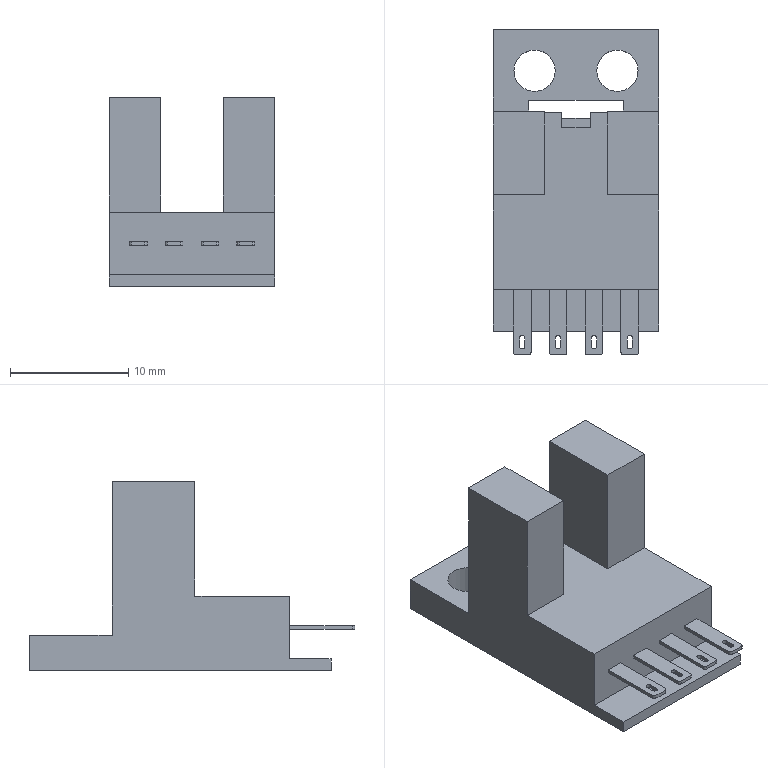Part | NX | 1 solid | 75 faces | box 14 x 27.5 x 16 mm | volume 2157 mm3 | plane 55 | cylinder 20 | commonest cylinder face diameters 0.4 x8 0.431 x8 3.5 x4